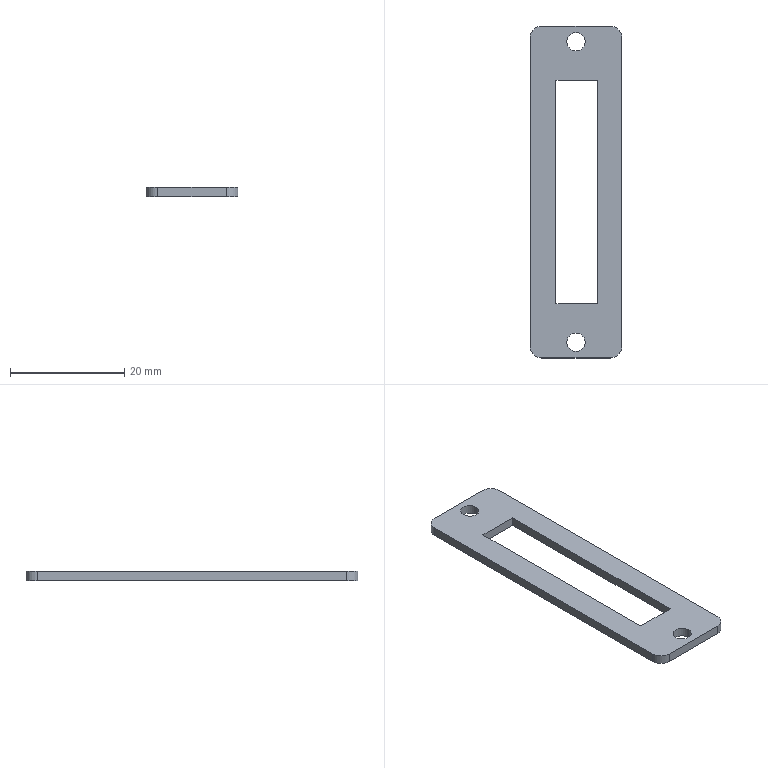Part | NX | features BREP 1 | 1 solid | 18 faces | box 16 x 58 x 1.6 mm | volume 998.284 mm3 | plane 10 | cylinder 8 | commonest cylinder face diameters 3.2 x4 4 x4
STEP:
#1=CARTESIAN_POINT('',(233.9,92.858,1.6));
#2=VERTEX_POINT('',#1);
#3=CARTESIAN_POINT('',(237.1,92.858,1.6));
#4=VERTEX_POINT('',#3);
#5=CARTESIAN_POINT('',(235.5,92.858,1.6));
#6=DIRECTION('',(0.,0.,1.));
#7=DIRECTION('',(1.,0.,0.));
#8=AXIS2_PLACEMENT_3D('',#5,#6,#7);
#9=CIRCLE('',#8,1.6);
#10=EDGE_CURVE('',#2,#4,#9,.T.);
#11=ORIENTED_EDGE('',*,*,#10,.T.);
#12=CARTESIAN_POINT('',(237.1,92.858,0.));
#13=VERTEX_POINT('',#12);
#14=CARTESIAN_POINT('',(237.1,92.858,1.6));
#15=DIRECTION('',(0.,0.,-1.));
#16=VECTOR('',#15,1000.);
#17=LINE('',#14,#16);
#18=EDGE_CURVE('',#13,#4,#17,.F.);
#19=ORIENTED_EDGE('',*,*,#18,.F.);
#20=CARTESIAN_POINT('',(233.9,92.858,0.));
#21=VERTEX_POINT('',#20);
#22=CARTESIAN_POINT('',(235.5,92.858,0.));
#23=DIRECTION('',(0.,0.,1.));
#24=DIRECTION('',(1.,0.,0.));
#25=AXIS2_PLACEMENT_3D('',#22,#23,#24);
#26=CIRCLE('',#25,1.6);
#27=EDGE_CURVE('',#21,#13,#26,.T.);
#28=ORIENTED_EDGE('',*,*,#27,.F.);
#29=CARTESIAN_POINT('',(233.9,92.858,1.6));
#30=DIRECTION('',(0.,0.,-1.));
#31=VECTOR('',#30,1000.);
#32=LINE('',#29,#31);
#33=EDGE_CURVE('',#21,#2,#32,.F.);
#34=ORIENTED_EDGE('',*,*,#33,.T.);
#35=EDGE_LOOP('',(#11,#19,#28,#34));
#36=FACE_BOUND('',#35,.T.);
#37=CARTESIAN_POINT('',(235.5,92.858,1.6));
#38=DIRECTION('',(0.,0.,-1.));
#39=DIRECTION('',(1.,0.,0.));
#40=AXIS2_PLACEMENT_3D('',#37,#38,#39);
#41=CYLINDRICAL_SURFACE('',#40,1.6);
#42=ADVANCED_FACE('',(#36),#41,.F.);
#43=CARTESIAN_POINT('',(233.9,40.358,1.6));
#44=VERTEX_POINT('',#43);
#45=CARTESIAN_POINT('',(237.1,40.358,1.6));
#46=VERTEX_POINT('',#45);
#47=CARTESIAN_POINT('',(235.5,40.358,1.6));
#48=DIRECTION('',(0.,0.,1.));
#49=DIRECTION('',(1.,0.,0.));
#50=AXIS2_PLACEMENT_3D('',#47,#48,#49);
#51=CIRCLE('',#50,1.6);
#52=EDGE_CURVE('',#44,#46,#51,.T.);
#53=ORIENTED_EDGE('',*,*,#52,.T.);
#54=CARTESIAN_POINT('',(237.1,40.358,0.));
#55=VERTEX_POINT('',#54);
#56=CARTESIAN_POINT('',(237.1,40.358,1.6));
#57=DIRECTION('',(0.,0.,-1.));
#58=VECTOR('',#57,1000.);
#59=LINE('',#56,#58);
#60=EDGE_CURVE('',#55,#46,#59,.F.);
#61=ORIENTED_EDGE('',*,*,#60,.F.);
#62=CARTESIAN_POINT('',(233.9,40.358,0.));
#63=VERTEX_POINT('',#62);
#64=CARTESIAN_POINT('',(235.5,40.358,0.));
#65=DIRECTION('',(0.,0.,1.));
#66=DIRECTION('',(1.,0.,0.));
#67=AXIS2_PLACEMENT_3D('',#64,#65,#66);
#68=CIRCLE('',#67,1.6);
#69=EDGE_CURVE('',#63,#55,#68,.T.);
#70=ORIENTED_EDGE('',*,*,#69,.F.);
#71=CARTESIAN_POINT('',(233.9,40.358,1.6));
#72=DIRECTION('',(0.,0.,-1.));
#73=VECTOR('',#72,1000.);
#74=LINE('',#71,#73);
#75=EDGE_CURVE('',#63,#44,#74,.F.);
#76=ORIENTED_EDGE('',*,*,#75,.T.);
#77=EDGE_LOOP('',(#53,#61,#70,#76));
#78=FACE_BOUND('',#77,.T.);
#79=CARTESIAN_POINT('',(235.5,40.358,1.6));
#80=DIRECTION('',(0.,0.,-1.));
#81=DIRECTION('',(1.,0.,0.));
#82=AXIS2_PLACEMENT_3D('',#79,#80,#81);
#83=CYLINDRICAL_SURFACE('',#82,1.6);
#84=ADVANCED_FACE('',(#78),#83,.F.);
#85=CARTESIAN_POINT('',(243.5,93.608,1.6));
#86=VERTEX_POINT('',#85);
#87=CARTESIAN_POINT('',(241.5,95.608,1.6));
#88=VERTEX_POINT('',#87);
#89=CARTESIAN_POINT('',(241.5,93.608,1.6));
#90=DIRECTION('',(0.,0.,1.));
#91=DIRECTION('',(-1.,0.,0.));
#92=AXIS2_PLACEMENT_3D('',#89,#90,#91);
#93=CIRCLE('',#92,2.);
#94=EDGE_CURVE('',#86,#88,#93,.T.);
#95=ORIENTED_EDGE('',*,*,#94,.T.);
#96=CARTESIAN_POINT('',(229.5,95.608,1.6));
#97=VERTEX_POINT('',#96);
#98=CARTESIAN_POINT('',(229.5,95.608,1.6));
#99=DIRECTION('',(-1.,0.,0.));
#100=VECTOR('',#99,1000.);
#101=LINE('',#98,#100);
#102=EDGE_CURVE('',#88,#97,#101,.T.);
#103=ORIENTED_EDGE('',*,*,#102,.T.);
#104=CARTESIAN_POINT('',(227.5,93.608,1.6));
#105=VERTEX_POINT('',#104);
#106=CARTESIAN_POINT('',(229.5,93.608,1.6));
#107=DIRECTION('',(0.,0.,1.));
#108=DIRECTION('',(1.,0.,0.));
#109=AXIS2_PLACEMENT_3D('',#106,#107,#108);
#110=CIRCLE('',#109,2.);
#111=EDGE_CURVE('',#97,#105,#110,.T.);
#112=ORIENTED_EDGE('',*,*,#111,.T.);
#113=CARTESIAN_POINT('',(227.5,39.608,1.6));
#114=VERTEX_POINT('',#113);
#115=CARTESIAN_POINT('',(227.5,93.608,1.6));
#116=DIRECTION('',(0.,-1.,0.));
#117=VECTOR('',#116,1000.);
#118=LINE('',#115,#117);
#119=EDGE_CURVE('',#105,#114,#118,.T.);
#120=ORIENTED_EDGE('',*,*,#119,.T.);
#121=CARTESIAN_POINT('',(229.5,37.608,1.6));
#122=VERTEX_POINT('',#121);
#123=CARTESIAN_POINT('',(229.5,39.608,1.6));
#124=DIRECTION('',(0.,0.,1.));
#125=DIRECTION('',(1.,0.,0.));
#126=AXIS2_PLACEMENT_3D('',#123,#124,#125);
#127=CIRCLE('',#126,2.);
#128=EDGE_CURVE('',#114,#122,#127,.T.);
#129=ORIENTED_EDGE('',*,*,#128,.T.);
#130=CARTESIAN_POINT('',(241.5,37.608,1.6));
#131=VERTEX_POINT('',#130);
#132=CARTESIAN_POINT('',(229.5,37.608,1.6));
#133=DIRECTION('',(1.,0.,0.));
#134=VECTOR('',#133,1000.);
#135=LINE('',#132,#134);
#136=EDGE_CURVE('',#122,#131,#135,.T.);
#137=ORIENTED_EDGE('',*,*,#136,.T.);
#138=CARTESIAN_POINT('',(243.5,39.608,1.6));
#139=VERTEX_POINT('',#138);
#140=CARTESIAN_POINT('',(241.5,39.608,1.6));
#141=DIRECTION('',(0.,0.,1.));
#142=DIRECTION('',(1.,0.,0.));
#143=AXIS2_PLACEMENT_3D('',#140,#141,#142);
#144=CIRCLE('',#143,2.);
#145=EDGE_CURVE('',#131,#139,#144,.T.);
#146=ORIENTED_EDGE('',*,*,#145,.T.);
#147=CARTESIAN_POINT('',(243.5,93.608,1.6));
#148=DIRECTION('',(0.,1.,0.));
#149=VECTOR('',#148,1000.);
#150=LINE('',#147,#149);
#151=EDGE_CURVE('',#139,#86,#150,.T.);
#152=ORIENTED_EDGE('',*,*,#151,.T.);
#153=EDGE_LOOP('',(#95,#103,#112,#120,#129,#137,#146,#152));
#154=FACE_BOUND('',#153,.T.);
#155=CARTESIAN_POINT('',(239.3,47.118,1.6));
#156=VERTEX_POINT('',#155);
#157=CARTESIAN_POINT('',(232.,47.118,1.6));
#158=VERTEX_POINT('',#157);
#159=CARTESIAN_POINT('',(239.3,47.118,1.6));
#160=DIRECTION('',(-1.,0.,0.));
#161=VECTOR('',#160,1000.);
#162=LINE('',#159,#161);
#163=EDGE_CURVE('',#156,#158,#162,.T.);
#164=ORIENTED_EDGE('',*,*,#163,.T.);
#165=CARTESIAN_POINT('',(232.,86.098,1.6));
#166=VERTEX_POINT('',#165);
#167=CARTESIAN_POINT('',(232.,47.118,1.6));
#168=DIRECTION('',(0.,1.,0.));
#169=VECTOR('',#168,1000.);
#170=LINE('',#167,#169);
#171=EDGE_CURVE('',#158,#166,#170,.T.);
#172=ORIENTED_EDGE('',*,*,#171,.T.);
#173=CARTESIAN_POINT('',(239.3,86.098,1.6));
#174=VERTEX_POINT('',#173);
#175=CARTESIAN_POINT('',(232.,86.098,1.6));
#176=DIRECTION('',(1.,0.,0.));
#177=VECTOR('',#176,1000.);
#178=LINE('',#175,#177);
#179=EDGE_CURVE('',#166,#174,#178,.T.);
#180=ORIENTED_EDGE('',*,*,#179,.T.);
#181=CARTESIAN_POINT('',(239.3,86.098,1.6));
#182=DIRECTION('',(0.,-1.,0.));
#183=VECTOR('',#182,1000.);
#184=LINE('',#181,#183);
#185=EDGE_CURVE('',#174,#156,#184,.T.);
#186=ORIENTED_EDGE('',*,*,#185,.T.);
#187=EDGE_LOOP('',(#164,#172,#180,#186));
#188=FACE_BOUND('',#187,.T.);
#189=ORIENTED_EDGE('',*,*,#52,.F.);
#190=CARTESIAN_POINT('',(235.5,40.358,1.6));
#191=DIRECTION('',(0.,0.,1.));
#192=DIRECTION('',(1.,0.,0.));
#193=AXIS2_PLACEMENT_3D('',#190,#191,#192);
#194=CIRCLE('',#193,1.6);
#195=EDGE_CURVE('',#46,#44,#194,.T.);
#196=ORIENTED_EDGE('',*,*,#195,.F.);
#197=EDGE_LOOP('',(#189,#196));
#198=FACE_BOUND('',#197,.T.);
#199=ORIENTED_EDGE('',*,*,#10,.F.);
#200=CARTESIAN_POINT('',(235.5,92.858,1.6));
#201=DIRECTION('',(0.,0.,1.));
#202=DIRECTION('',(1.,0.,0.));
#203=AXIS2_PLACEMENT_3D('',#200,#201,#202);
#204=CIRCLE('',#203,1.6);
#205=EDGE_CURVE('',#4,#2,#204,.T.);
#206=ORIENTED_EDGE('',*,*,#205,.F.);
#207=EDGE_LOOP('',(#199,#206));
#208=FACE_BOUND('',#207,.T.);
#209=CARTESIAN_POINT('',(241.5,93.608,1.6));
#210=DIRECTION('',(0.,0.,-1.));
#211=DIRECTION('',(0.,1.,0.));
#212=AXIS2_PLACEMENT_3D('',#209,#210,#211);
#213=PLANE('',#212);
#214=ADVANCED_FACE('',(#154,#188,#198,#208),#213,.F.);
#215=CARTESIAN_POINT('',(243.5,93.608,0.));
#216=VERTEX_POINT('',#215);
#217=CARTESIAN_POINT('',(241.5,95.608,0.));
#218=VERTEX_POINT('',#217);
#219=CARTESIAN_POINT('',(241.5,93.608,0.));
#220=DIRECTION('',(0.,0.,1.));
#221=DIRECTION('',(-1.,0.,0.));
#222=AXIS2_PLACEMENT_3D('',#219,#220,#221);
#223=CIRCLE('',#222,2.);
#224=EDGE_CURVE('',#216,#218,#223,.T.);
#225=ORIENTED_EDGE('',*,*,#224,.F.);
#226=CARTESIAN_POINT('',(243.5,39.608,0.));
#227=VERTEX_POINT('',#226);
#228=CARTESIAN_POINT('',(243.5,93.608,0.));
#229=DIRECTION('',(0.,1.,0.));
#230=VECTOR('',#229,1000.);
#231=LINE('',#228,#230);
#232=EDGE_CURVE('',#227,#216,#231,.T.);
#233=ORIENTED_EDGE('',*,*,#232,.F.);
#234=CARTESIAN_POINT('',(241.5,37.608,0.));
#235=VERTEX_POINT('',#234);
#236=CARTESIAN_POINT('',(241.5,39.608,0.));
#237=DIRECTION('',(0.,0.,1.));
#238=DIRECTION('',(1.,0.,0.));
#239=AXIS2_PLACEMENT_3D('',#236,#237,#238);
#240=CIRCLE('',#239,2.);
#241=EDGE_CURVE('',#235,#227,#240,.T.);
#242=ORIENTED_EDGE('',*,*,#241,.F.);
#243=CARTESIAN_POINT('',(229.5,37.608,0.));
#244=VERTEX_POINT('',#243);
#245=CARTESIAN_POINT('',(229.5,37.608,0.));
#246=DIRECTION('',(1.,0.,0.));
#247=VECTOR('',#246,1000.);
#248=LINE('',#245,#247);
#249=EDGE_CURVE('',#244,#235,#248,.T.);
#250=ORIENTED_EDGE('',*,*,#249,.F.);
#251=CARTESIAN_POINT('',(227.5,39.608,0.));
#252=VERTEX_POINT('',#251);
#253=CARTESIAN_POINT('',(229.5,39.608,0.));
#254=DIRECTION('',(0.,0.,1.));
#255=DIRECTION('',(1.,0.,0.));
#256=AXIS2_PLACEMENT_3D('',#253,#254,#255);
#257=CIRCLE('',#256,2.);
#258=EDGE_CURVE('',#252,#244,#257,.T.);
#259=ORIENTED_EDGE('',*,*,#258,.F.);
#260=CARTESIAN_POINT('',(227.5,93.608,0.));
#261=VERTEX_POINT('',#260);
#262=CARTESIAN_POINT('',(227.5,93.608,0.));
#263=DIRECTION('',(0.,-1.,0.));
#264=VECTOR('',#263,1000.);
#265=LINE('',#262,#264);
#266=EDGE_CURVE('',#261,#252,#265,.T.);
#267=ORIENTED_EDGE('',*,*,#266,.F.);
#268=CARTESIAN_POINT('',(229.5,95.608,0.));
#269=VERTEX_POINT('',#268);
#270=CARTESIAN_POINT('',(229.5,93.608,0.));
#271=DIRECTION('',(0.,0.,1.));
#272=DIRECTION('',(1.,0.,0.));
#273=AXIS2_PLACEMENT_3D('',#270,#271,#272);
#274=CIRCLE('',#273,2.);
#275=EDGE_CURVE('',#269,#261,#274,.T.);
#276=ORIENTED_EDGE('',*,*,#275,.F.);
#277=CARTESIAN_POINT('',(229.5,95.608,0.));
#278=DIRECTION('',(-1.,0.,0.));
#279=VECTOR('',#278,1000.);
#280=LINE('',#277,#279);
#281=EDGE_CURVE('',#218,#269,#280,.T.);
#282=ORIENTED_EDGE('',*,*,#281,.F.);
#283=EDGE_LOOP('',(#225,#233,#242,#250,#259,#267,#276,#282));
#284=FACE_BOUND('',#283,.T.);
#285=CARTESIAN_POINT('',(232.,47.118,0.));
#286=VERTEX_POINT('',#285);
#287=CARTESIAN_POINT('',(232.,86.098,0.));
#288=VERTEX_POINT('',#287);
#289=CARTESIAN_POINT('',(232.,47.118,0.));
#290=DIRECTION('',(0.,1.,0.));
#291=VECTOR('',#290,1000.);
#292=LINE('',#289,#291);
#293=EDGE_CURVE('',#286,#288,#292,.T.);
#294=ORIENTED_EDGE('',*,*,#293,.F.);
#295=CARTESIAN_POINT('',(239.3,47.118,0.));
#296=VERTEX_POINT('',#295);
#297=CARTESIAN_POINT('',(239.3,47.118,0.));
#298=DIRECTION('',(-1.,0.,0.));
#299=VECTOR('',#298,1000.);
#300=LINE('',#297,#299);
#301=EDGE_CURVE('',#296,#286,#300,.T.);
#302=ORIENTED_EDGE('',*,*,#301,.F.);
#303=CARTESIAN_POINT('',(239.3,86.098,0.));
#304=VERTEX_POINT('',#303);
#305=CARTESIAN_POINT('',(239.3,86.098,0.));
#306=DIRECTION('',(0.,-1.,0.));
#307=VECTOR('',#306,1000.);
#308=LINE('',#305,#307);
#309=EDGE_CURVE('',#304,#296,#308,.T.);
#310=ORIENTED_EDGE('',*,*,#309,.F.);
#311=CARTESIAN_POINT('',(232.,86.098,0.));
#312=DIRECTION('',(1.,0.,0.));
#313=VECTOR('',#312,1000.);
#314=LINE('',#311,#313);
#315=EDGE_CURVE('',#288,#304,#314,.T.);
#316=ORIENTED_EDGE('',*,*,#315,.F.);
#317=EDGE_LOOP('',(#294,#302,#310,#316));
#318=FACE_BOUND('',#317,.T.);
#319=ORIENTED_EDGE('',*,*,#69,.T.);
#320=CARTESIAN_POINT('',(235.5,40.358,0.));
#321=DIRECTION('',(0.,0.,1.));
#322=DIRECTION('',(1.,0.,0.));
#323=AXIS2_PLACEMENT_3D('',#320,#321,#322);
#324=CIRCLE('',#323,1.6);
#325=EDGE_CURVE('',#55,#63,#324,.T.);
#326=ORIENTED_EDGE('',*,*,#325,.T.);
#327=EDGE_LOOP('',(#319,#326));
#328=FACE_BOUND('',#327,.T.);
#329=ORIENTED_EDGE('',*,*,#27,.T.);
#330=CARTESIAN_POINT('',(235.5,92.858,0.));
#331=DIRECTION('',(0.,0.,1.));
#332=DIRECTION('',(1.,0.,0.));
#333=AXIS2_PLACEMENT_3D('',#330,#331,#332);
#334=CIRCLE('',#333,1.6);
#335=EDGE_CURVE('',#13,#21,#334,.T.);
#336=ORIENTED_EDGE('',*,*,#335,.T.);
#337=EDGE_LOOP('',(#329,#336));
#338=FACE_BOUND('',#337,.T.);
#339=CARTESIAN_POINT('',(241.5,93.608,0.));
#340=DIRECTION('',(0.,0.,-1.));
#341=DIRECTION('',(0.,1.,0.));
#342=AXIS2_PLACEMENT_3D('',#339,#340,#341);
#343=PLANE('',#342);
#344=ADVANCED_FACE('',(#284,#318,#328,#338),#343,.T.);
#345=ORIENTED_EDGE('',*,*,#224,.T.);
#346=CARTESIAN_POINT('',(241.5,95.608,1.6));
#347=DIRECTION('',(0.,0.,-1.));
#348=VECTOR('',#347,1000.);
#349=LINE('',#346,#348);
#350=EDGE_CURVE('',#88,#218,#349,.T.);
#351=ORIENTED_EDGE('',*,*,#350,.F.);
#352=ORIENTED_EDGE('',*,*,#94,.F.);
#353=CARTESIAN_POINT('',(243.5,93.608,1.6));
#354=DIRECTION('',(0.,0.,-1.));
#355=VECTOR('',#354,1000.);
#356=LINE('',#353,#355);
#357=EDGE_CURVE('',#86,#216,#356,.T.);
#358=ORIENTED_EDGE('',*,*,#357,.T.);
#359=EDGE_LOOP('',(#345,#351,#352,#358));
#360=FACE_BOUND('',#359,.T.);
#361=CARTESIAN_POINT('',(241.5,93.608,1.6));
#362=DIRECTION('',(0.,0.,-1.));
#363=DIRECTION('',(1.,0.,0.));
#364=AXIS2_PLACEMENT_3D('',#361,#362,#363);
#365=CYLINDRICAL_SURFACE('',#364,2.);
#366=ADVANCED_FACE('',(#360),#365,.T.);
#367=ORIENTED_EDGE('',*,*,#281,.T.);
#368=CARTESIAN_POINT('',(229.5,95.608,1.6));
#369=DIRECTION('',(0.,0.,-1.));
#370=VECTOR('',#369,1000.);
#371=LINE('',#368,#370);
#372=EDGE_CURVE('',#97,#269,#371,.T.);
#373=ORIENTED_EDGE('',*,*,#372,.F.);
#374=ORIENTED_EDGE('',*,*,#102,.F.);
#375=ORIENTED_EDGE('',*,*,#350,.T.);
#376=EDGE_LOOP('',(#367,#373,#374,#375));
#377=FACE_BOUND('',#376,.T.);
#378=CARTESIAN_POINT('',(229.5,95.608,1.6));
#379=DIRECTION('',(0.,-1.,0.));
#380=DIRECTION('',(0.,0.,1.));
#381=AXIS2_PLACEMENT_3D('',#378,#379,#380);
#382=PLANE('',#381);
#383=ADVANCED_FACE('',(#377),#382,.F.);
#384=ORIENTED_EDGE('',*,*,#275,.T.);
#385=CARTESIAN_POINT('',(227.5,93.608,1.6));
#386=DIRECTION('',(0.,0.,-1.));
#387=VECTOR('',#386,1000.);
#388=LINE('',#385,#387);
#389=EDGE_CURVE('',#105,#261,#388,.T.);
#390=ORIENTED_EDGE('',*,*,#389,.F.);
#391=ORIENTED_EDGE('',*,*,#111,.F.);
#392=ORIENTED_EDGE('',*,*,#372,.T.);
#393=EDGE_LOOP('',(#384,#390,#391,#392));
#394=FACE_BOUND('',#393,.T.);
#395=CARTESIAN_POINT('',(229.5,93.608,1.6));
#396=DIRECTION('',(0.,0.,-1.));
#397=DIRECTION('',(1.,0.,0.));
#398=AXIS2_PLACEMENT_3D('',#395,#396,#397);
#399=CYLINDRICAL_SURFACE('',#398,2.);
#400=ADVANCED_FACE('',(#394),#399,.T.);
#401=ORIENTED_EDGE('',*,*,#266,.T.);
#402=CARTESIAN_POINT('',(227.5,39.608,1.6));
#403=DIRECTION('',(0.,0.,-1.));
#404=VECTOR('',#403,1000.);
#405=LINE('',#402,#404);
#406=EDGE_CURVE('',#114,#252,#405,.T.);
#407=ORIENTED_EDGE('',*,*,#406,.F.);
#408=ORIENTED_EDGE('',*,*,#119,.F.);
#409=ORIENTED_EDGE('',*,*,#389,.T.);
#410=EDGE_LOOP('',(#401,#407,#408,#409));
#411=FACE_BOUND('',#410,.T.);
#412=CARTESIAN_POINT('',(227.5,93.608,1.6));
#413=DIRECTION('',(1.,0.,0.));
#414=DIRECTION('',(0.,-1.,0.));
#415=AXIS2_PLACEMENT_3D('',#412,#413,#414);
#416=PLANE('',#415);
#417=ADVANCED_FACE('',(#411),#416,.F.);
#418=ORIENTED_EDGE('',*,*,#258,.T.);
#419=CARTESIAN_POINT('',(229.5,37.608,1.6));
#420=DIRECTION('',(0.,0.,-1.));
#421=VECTOR('',#420,1000.);
#422=LINE('',#419,#421);
#423=EDGE_CURVE('',#122,#244,#422,.T.);
#424=ORIENTED_EDGE('',*,*,#423,.F.);
#425=ORIENTED_EDGE('',*,*,#128,.F.);
#426=ORIENTED_EDGE('',*,*,#406,.T.);
#427=EDGE_LOOP('',(#418,#424,#425,#426));
#428=FACE_BOUND('',#427,.T.);
#429=CARTESIAN_POINT('',(229.5,39.608,1.6));
#430=DIRECTION('',(0.,0.,-1.));
#431=DIRECTION('',(1.,0.,0.));
#432=AXIS2_PLACEMENT_3D('',#429,#430,#431);
#433=CYLINDRICAL_SURFACE('',#432,2.);
#434=ADVANCED_FACE('',(#428),#433,.T.);
#435=ORIENTED_EDGE('',*,*,#249,.T.);
#436=CARTESIAN_POINT('',(241.5,37.608,1.6));
#437=DIRECTION('',(0.,0.,-1.));
#438=VECTOR('',#437,1000.);
#439=LINE('',#436,#438);
#440=EDGE_CURVE('',#131,#235,#439,.T.);
#441=ORIENTED_EDGE('',*,*,#440,.F.);
#442=ORIENTED_EDGE('',*,*,#136,.F.);
#443=ORIENTED_EDGE('',*,*,#423,.T.);
#444=EDGE_LOOP('',(#435,#441,#442,#443));
#445=FACE_BOUND('',#444,.T.);
#446=CARTESIAN_POINT('',(229.5,37.608,1.6));
#447=DIRECTION('',(0.,1.,0.));
#448=DIRECTION('',(-1.,0.,0.));
#449=AXIS2_PLACEMENT_3D('',#446,#447,#448);
#450=PLANE('',#449);
#451=ADVANCED_FACE('',(#445),#450,.F.);
#452=ORIENTED_EDGE('',*,*,#241,.T.);
#453=CARTESIAN_POINT('',(243.5,39.608,1.6));
#454=DIRECTION('',(0.,0.,-1.));
#455=VECTOR('',#454,1000.);
#456=LINE('',#453,#455);
#457=EDGE_CURVE('',#139,#227,#456,.T.);
#458=ORIENTED_EDGE('',*,*,#457,.F.);
#459=ORIENTED_EDGE('',*,*,#145,.F.);
#460=ORIENTED_EDGE('',*,*,#440,.T.);
#461=EDGE_LOOP('',(#452,#458,#459,#460));
#462=FACE_BOUND('',#461,.T.);
#463=CARTESIAN_POINT('',(241.5,39.608,1.6));
#464=DIRECTION('',(0.,0.,-1.));
#465=DIRECTION('',(1.,0.,0.));
#466=AXIS2_PLACEMENT_3D('',#463,#464,#465);
#467=CYLINDRICAL_SURFACE('',#466,2.);
#468=ADVANCED_FACE('',(#462),#467,.T.);
#469=ORIENTED_EDGE('',*,*,#232,.T.);
#470=ORIENTED_EDGE('',*,*,#357,.F.);
#471=ORIENTED_EDGE('',*,*,#151,.F.);
#472=ORIENTED_EDGE('',*,*,#457,.T.);
#473=EDGE_LOOP('',(#469,#470,#471,#472));
#474=FACE_BOUND('',#473,.T.);
#475=CARTESIAN_POINT('',(243.5,93.608,1.6));
#476=DIRECTION('',(-1.,0.,0.));
#477=DIRECTION('',(0.,0.,-1.));
#478=AXIS2_PLACEMENT_3D('',#475,#476,#477);
#479=PLANE('',#478);
#480=ADVANCED_FACE('',(#474),#479,.F.);
#481=ORIENTED_EDGE('',*,*,#60,.T.);
#482=ORIENTED_EDGE('',*,*,#195,.T.);
#483=ORIENTED_EDGE('',*,*,#75,.F.);
#484=ORIENTED_EDGE('',*,*,#325,.F.);
#485=EDGE_LOOP('',(#481,#482,#483,#484));
#486=FACE_BOUND('',#485,.T.);
#487=CARTESIAN_POINT('',(235.5,40.358,1.6));
#488=DIRECTION('',(0.,0.,-1.));
#489=DIRECTION('',(1.,0.,0.));
#490=AXIS2_PLACEMENT_3D('',#487,#488,#489);
#491=CYLINDRICAL_SURFACE('',#490,1.6);
#492=ADVANCED_FACE('',(#486),#491,.F.);
#493=ORIENTED_EDGE('',*,*,#18,.T.);
#494=ORIENTED_EDGE('',*,*,#205,.T.);
#495=ORIENTED_EDGE('',*,*,#33,.F.);
#496=ORIENTED_EDGE('',*,*,#335,.F.);
#497=EDGE_LOOP('',(#493,#494,#495,#496));
#498=FACE_BOUND('',#497,.T.);
#499=CARTESIAN_POINT('',(235.5,92.858,1.6));
#500=DIRECTION('',(0.,0.,-1.));
#501=DIRECTION('',(1.,0.,0.));
#502=AXIS2_PLACEMENT_3D('',#499,#500,#501);
#503=CYLINDRICAL_SURFACE('',#502,1.6);
#504=ADVANCED_FACE('',(#498),#503,.F.);
#505=ORIENTED_EDGE('',*,*,#293,.T.);
#506=CARTESIAN_POINT('',(232.,86.098,1.6));
#507=DIRECTION('',(0.,0.,-1.));
#508=VECTOR('',#507,1000.);
#509=LINE('',#506,#508);
#510=EDGE_CURVE('',#166,#288,#509,.T.);
#511=ORIENTED_EDGE('',*,*,#510,.F.);
#512=ORIENTED_EDGE('',*,*,#171,.F.);
#513=CARTESIAN_POINT('',(232.,47.118,1.6));
#514=DIRECTION('',(0.,0.,-1.));
#515=VECTOR('',#514,1000.);
#516=LINE('',#513,#515);
#517=EDGE_CURVE('',#158,#286,#516,.T.);
#518=ORIENTED_EDGE('',*,*,#517,.T.);
#519=EDGE_LOOP('',(#505,#511,#512,#518));
#520=FACE_BOUND('',#519,.T.);
#521=CARTESIAN_POINT('',(232.,47.118,1.6));
#522=DIRECTION('',(-1.,0.,0.));
#523=DIRECTION('',(0.,0.,-1.));
#524=AXIS2_PLACEMENT_3D('',#521,#522,#523);
#525=PLANE('',#524);
#526=ADVANCED_FACE('',(#520),#525,.F.);
#527=ORIENTED_EDGE('',*,*,#301,.T.);
#528=ORIENTED_EDGE('',*,*,#517,.F.);
#529=ORIENTED_EDGE('',*,*,#163,.F.);
#530=CARTESIAN_POINT('',(239.3,47.118,1.6));
#531=DIRECTION('',(0.,0.,-1.));
#532=VECTOR('',#531,1000.);
#533=LINE('',#530,#532);
#534=EDGE_CURVE('',#156,#296,#533,.T.);
#535=ORIENTED_EDGE('',*,*,#534,.T.);
#536=EDGE_LOOP('',(#527,#528,#529,#535));
#537=FACE_BOUND('',#536,.T.);
#538=CARTESIAN_POINT('',(239.3,47.118,1.6));
#539=DIRECTION('',(0.,-1.,0.));
#540=DIRECTION('',(0.,0.,1.));
#541=AXIS2_PLACEMENT_3D('',#538,#539,#540);
#542=PLANE('',#541);
#543=ADVANCED_FACE('',(#537),#542,.F.);
#544=ORIENTED_EDGE('',*,*,#309,.T.);
#545=ORIENTED_EDGE('',*,*,#534,.F.);
#546=ORIENTED_EDGE('',*,*,#185,.F.);
#547=CARTESIAN_POINT('',(239.3,86.098,1.6));
#548=DIRECTION('',(0.,0.,-1.));
#549=VECTOR('',#548,1000.);
#550=LINE('',#547,#549);
#551=EDGE_CURVE('',#174,#304,#550,.T.);
#552=ORIENTED_EDGE('',*,*,#551,.T.);
#553=EDGE_LOOP('',(#544,#545,#546,#552));
#554=FACE_BOUND('',#553,.T.);
#555=CARTESIAN_POINT('',(239.3,86.098,1.6));
#556=DIRECTION('',(1.,0.,0.));
#557=DIRECTION('',(0.,-1.,0.));
#558=AXIS2_PLACEMENT_3D('',#555,#556,#557);
#559=PLANE('',#558);
#560=ADVANCED_FACE('',(#554),#559,.F.);
#561=ORIENTED_EDGE('',*,*,#315,.T.);
#562=ORIENTED_EDGE('',*,*,#551,.F.);
#563=ORIENTED_EDGE('',*,*,#179,.F.);
#564=ORIENTED_EDGE('',*,*,#510,.T.);
#565=EDGE_LOOP('',(#561,#562,#563,#564));
#566=FACE_BOUND('',#565,.T.);
#567=CARTESIAN_POINT('',(232.,86.098,1.6));
#568=DIRECTION('',(0.,1.,0.));
#569=DIRECTION('',(-1.,0.,0.));
#570=AXIS2_PLACEMENT_3D('',#567,#568,#569);
#571=PLANE('',#570);
#572=ADVANCED_FACE('',(#566),#571,.F.);
#573=CLOSED_SHELL('',(#42,#84,#214,#344,#366,#383,#400,#417,#434,#451,#468,#480,#492,#504,#526,#543,#560,#572));
#574=MANIFOLD_SOLID_BREP('',#573);
#575=(LENGTH_UNIT()NAMED_UNIT(*)SI_UNIT(.MILLI.,.METRE.));
#576=UNCERTAINTY_MEASURE_WITH_UNIT(LENGTH_MEASURE(0.00001),#575,'','');
#577=(NAMED_UNIT(*)PLANE_ANGLE_UNIT()SI_UNIT($,.RADIAN.));
#578=(NAMED_UNIT(*)SI_UNIT($,.STERADIAN.)SOLID_ANGLE_UNIT());
#579=(GEOMETRIC_REPRESENTATION_CONTEXT(3)GLOBAL_UNCERTAINTY_ASSIGNED_CONTEXT((#576))GLOBAL_UNIT_ASSIGNED_CONTEXT((#575,#577,#578))REPRESENTATION_CONTEXT('',''));
#580=ADVANCED_BREP_SHAPE_REPRESENTATION('',(#574),#579);